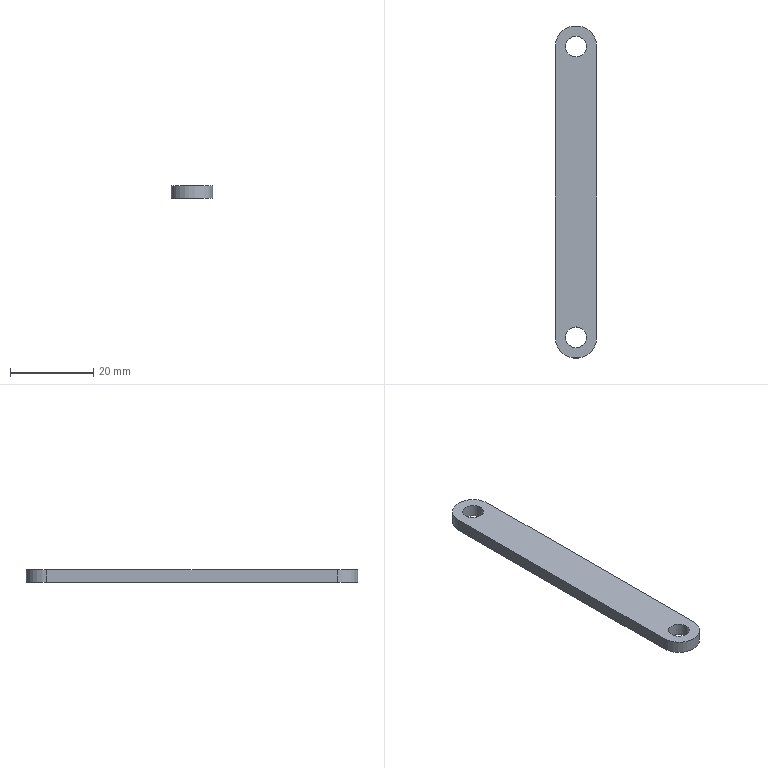Part | STEP file | 1-28.6 | 1 solid | 8 faces | box 10 x 80 x 3 mm | volume 2218 mm3 | plane 4 | cylinder 4 | commonest cylinder face diameters 5 x2 10 x2
STEP:
#1=CARTESIAN_POINT('',(0.,0.,0.));
#2=DIRECTION('',(0.,0.,1.));
#3=DIRECTION('',(1.,0.,0.));
#4=AXIS2_PLACEMENT_3D('',#1,#2,#3);
#5=CARTESIAN_POINT('',(-5.,0.,0.));
#6=VERTEX_POINT('',#5);
#7=CARTESIAN_POINT('',(5.,0.,0.));
#8=VERTEX_POINT('',#7);
#9=CARTESIAN_POINT('',(0.,0.,0.));
#10=DIRECTION('',(0.,0.,1.));
#11=DIRECTION('',(-1.,0.,0.));
#12=AXIS2_PLACEMENT_3D('',#9,#10,#11);
#13=CIRCLE('',#12,5.);
#14=CARTESIAN_POINT('',(-35.,35.,0.));
#15=DIRECTION('',(0.,0.,1.));
#16=DIRECTION('',(0.,1.,0.));
#17=AXIS2_PLACEMENT_3D('',#14,#15,#16);
#18=PLANE('',#17);
#19=CARTESIAN_POINT('',(-35.,-35.));
#20=DIRECTION('',(0.,1.));
#21=AXIS2_PLACEMENT_2D('',#19,#20);
#22=CIRCLE('',#21,5.);
#23=(GEOMETRIC_REPRESENTATION_CONTEXT(2)PARAMETRIC_REPRESENTATION_CONTEXT()REPRESENTATION_CONTEXT('',''));
#24=DEFINITIONAL_REPRESENTATION('',(#22),#23);
#25=PCURVE('',#18,#24);
#26=CARTESIAN_POINT('',(0.,0.,0.));
#27=DIRECTION('',(0.,0.,-1.));
#28=DIRECTION('',(-1.,0.,0.));
#29=AXIS2_PLACEMENT_3D('',#26,#27,#28);
#30=CYLINDRICAL_SURFACE('',#29,5.);
#31=CARTESIAN_POINT('',(6.283,0.));
#32=DIRECTION('',(-1.,0.));
#33=VECTOR('',#32,1.);
#34=LINE('',#31,#33);
#35=(GEOMETRIC_REPRESENTATION_CONTEXT(2)PARAMETRIC_REPRESENTATION_CONTEXT()REPRESENTATION_CONTEXT('',''));
#36=DEFINITIONAL_REPRESENTATION('',(#34),#35);
#37=PCURVE('',#30,#36);
#38=SURFACE_CURVE('',#13,(#25,#37),.PCURVE_S1.);
#39=EDGE_CURVE('',#6,#8,#38,.T.);
#40=ORIENTED_EDGE('',*,*,#39,.T.);
#41=CARTESIAN_POINT('',(5.,70.,0.));
#42=VERTEX_POINT('',#41);
#43=CARTESIAN_POINT('',(5.,0.,0.));
#44=DIRECTION('',(0.,1.,0.));
#45=VECTOR('',#44,1.);
#46=LINE('',#43,#45);
#47=CARTESIAN_POINT('',(-35.,-40.));
#48=DIRECTION('',(1.,0.));
#49=VECTOR('',#48,1.);
#50=LINE('',#47,#49);
#51=(GEOMETRIC_REPRESENTATION_CONTEXT(2)PARAMETRIC_REPRESENTATION_CONTEXT()REPRESENTATION_CONTEXT('',''));
#52=DEFINITIONAL_REPRESENTATION('',(#50),#51);
#53=PCURVE('',#18,#52);
#54=CARTESIAN_POINT('',(5.,35.,-1.5));
#55=DIRECTION('',(-1.,0.,0.));
#56=DIRECTION('',(0.,1.,0.));
#57=AXIS2_PLACEMENT_3D('',#54,#55,#56);
#58=PLANE('',#57);
#59=CARTESIAN_POINT('',(-35.,-1.5));
#60=DIRECTION('',(1.,0.));
#61=VECTOR('',#60,1.);
#62=LINE('',#59,#61);
#63=(GEOMETRIC_REPRESENTATION_CONTEXT(2)PARAMETRIC_REPRESENTATION_CONTEXT()REPRESENTATION_CONTEXT('',''));
#64=DEFINITIONAL_REPRESENTATION('',(#62),#63);
#65=PCURVE('',#58,#64);
#66=SURFACE_CURVE('',#46,(#53,#65),.PCURVE_S1.);
#67=EDGE_CURVE('',#8,#42,#66,.T.);
#68=ORIENTED_EDGE('',*,*,#67,.T.);
#69=CARTESIAN_POINT('',(-5.,70.,0.));
#70=VERTEX_POINT('',#69);
#71=CARTESIAN_POINT('',(0.,70.,0.));
#72=DIRECTION('',(0.,0.,1.));
#73=DIRECTION('',(1.,0.,0.));
#74=AXIS2_PLACEMENT_3D('',#71,#72,#73);
#75=CIRCLE('',#74,5.);
#76=CARTESIAN_POINT('',(35.,-35.));
#77=DIRECTION('',(0.,-1.));
#78=AXIS2_PLACEMENT_2D('',#76,#77);
#79=CIRCLE('',#78,5.);
#80=(GEOMETRIC_REPRESENTATION_CONTEXT(2)PARAMETRIC_REPRESENTATION_CONTEXT()REPRESENTATION_CONTEXT('',''));
#81=DEFINITIONAL_REPRESENTATION('',(#79),#80);
#82=PCURVE('',#18,#81);
#83=CARTESIAN_POINT('',(0.,70.,0.));
#84=DIRECTION('',(0.,0.,-1.));
#85=DIRECTION('',(1.,0.,0.));
#86=AXIS2_PLACEMENT_3D('',#83,#84,#85);
#87=CYLINDRICAL_SURFACE('',#86,5.);
#88=CARTESIAN_POINT('',(6.283,0.));
#89=DIRECTION('',(-1.,0.));
#90=VECTOR('',#89,1.);
#91=LINE('',#88,#90);
#92=(GEOMETRIC_REPRESENTATION_CONTEXT(2)PARAMETRIC_REPRESENTATION_CONTEXT()REPRESENTATION_CONTEXT('',''));
#93=DEFINITIONAL_REPRESENTATION('',(#91),#92);
#94=PCURVE('',#87,#93);
#95=SURFACE_CURVE('',#75,(#82,#94),.PCURVE_S1.);
#96=EDGE_CURVE('',#42,#70,#95,.T.);
#97=ORIENTED_EDGE('',*,*,#96,.T.);
#98=CARTESIAN_POINT('',(-5.,70.,0.));
#99=DIRECTION('',(0.,-1.,0.));
#100=VECTOR('',#99,1.);
#101=LINE('',#98,#100);
#102=CARTESIAN_POINT('',(35.,-30.));
#103=DIRECTION('',(-1.,0.));
#104=VECTOR('',#103,1.);
#105=LINE('',#102,#104);
#106=(GEOMETRIC_REPRESENTATION_CONTEXT(2)PARAMETRIC_REPRESENTATION_CONTEXT()REPRESENTATION_CONTEXT('',''));
#107=DEFINITIONAL_REPRESENTATION('',(#105),#106);
#108=PCURVE('',#18,#107);
#109=CARTESIAN_POINT('',(-5.,35.,-1.5));
#110=DIRECTION('',(1.,0.,0.));
#111=DIRECTION('',(0.,-1.,0.));
#112=AXIS2_PLACEMENT_3D('',#109,#110,#111);
#113=PLANE('',#112);
#114=CARTESIAN_POINT('',(-35.,-1.5));
#115=DIRECTION('',(1.,0.));
#116=VECTOR('',#115,1.);
#117=LINE('',#114,#116);
#118=(GEOMETRIC_REPRESENTATION_CONTEXT(2)PARAMETRIC_REPRESENTATION_CONTEXT()REPRESENTATION_CONTEXT('',''));
#119=DEFINITIONAL_REPRESENTATION('',(#117),#118);
#120=PCURVE('',#113,#119);
#121=SURFACE_CURVE('',#101,(#108,#120),.PCURVE_S1.);
#122=EDGE_CURVE('',#70,#6,#121,.T.);
#123=ORIENTED_EDGE('',*,*,#122,.T.);
#124=EDGE_LOOP('',(#40,#68,#97,#123));
#125=FACE_BOUND('',#124,.T.);
#126=CARTESIAN_POINT('',(0.,2.5,0.));
#127=VERTEX_POINT('',#126);
#128=CARTESIAN_POINT('',(0.,0.,0.));
#129=DIRECTION('',(0.,0.,-1.));
#130=DIRECTION('',(0.,1.,0.));
#131=AXIS2_PLACEMENT_3D('',#128,#129,#130);
#132=CIRCLE('',#131,2.5);
#133=CARTESIAN_POINT('',(-32.5,-35.));
#134=CARTESIAN_POINT('',(-32.5,-39.33));
#135=CARTESIAN_POINT('',(-36.25,-37.165));
#136=CARTESIAN_POINT('',(-40.,-35.));
#137=CARTESIAN_POINT('',(-36.25,-32.835));
#138=CARTESIAN_POINT('',(-32.5,-30.67));
#139=CARTESIAN_POINT('',(-32.5,-35.));
#140=(BOUNDED_CURVE()B_SPLINE_CURVE(2,(#133,#134,#135,#136,#137,#138,#139),.UNSPECIFIED.,.T.,.F.)B_SPLINE_CURVE_WITH_KNOTS((1,2,2,2,2,1),(-2.094,0.,2.094,4.189,6.283,8.378),.UNSPECIFIED.)CURVE()GEOMETRIC_REPRESENTATION_ITEM()RATIONAL_B_SPLINE_CURVE((1.,0.5,1.,0.5,1.,0.5,1.))REPRESENTATION_ITEM(''));
#141=(GEOMETRIC_REPRESENTATION_CONTEXT(2)PARAMETRIC_REPRESENTATION_CONTEXT()REPRESENTATION_CONTEXT('',''));
#142=DEFINITIONAL_REPRESENTATION('',(#140),#141);
#143=PCURVE('',#18,#142);
#144=CARTESIAN_POINT('',(0.,0.,0.));
#145=DIRECTION('',(0.,0.,-1.));
#146=DIRECTION('',(0.,1.,0.));
#147=AXIS2_PLACEMENT_3D('',#144,#145,#146);
#148=CYLINDRICAL_SURFACE('',#147,2.5);
#149=CARTESIAN_POINT('',(0.,0.));
#150=DIRECTION('',(1.,0.));
#151=VECTOR('',#150,1.);
#152=LINE('',#149,#151);
#153=(GEOMETRIC_REPRESENTATION_CONTEXT(2)PARAMETRIC_REPRESENTATION_CONTEXT()REPRESENTATION_CONTEXT('',''));
#154=DEFINITIONAL_REPRESENTATION('',(#152),#153);
#155=PCURVE('',#148,#154);
#156=SURFACE_CURVE('',#132,(#143,#155),.PCURVE_S1.);
#157=EDGE_CURVE('',#127,#127,#156,.T.);
#158=ORIENTED_EDGE('',*,*,#157,.T.);
#159=EDGE_LOOP('',(#158));
#160=FACE_BOUND('',#159,.T.);
#161=CARTESIAN_POINT('',(0.,72.5,0.));
#162=VERTEX_POINT('',#161);
#163=CARTESIAN_POINT('',(0.,70.,0.));
#164=DIRECTION('',(0.,0.,-1.));
#165=DIRECTION('',(0.,1.,0.));
#166=AXIS2_PLACEMENT_3D('',#163,#164,#165);
#167=CIRCLE('',#166,2.5);
#168=CARTESIAN_POINT('',(37.5,-35.));
#169=CARTESIAN_POINT('',(37.5,-39.33));
#170=CARTESIAN_POINT('',(33.75,-37.165));
#171=CARTESIAN_POINT('',(30.,-35.));
#172=CARTESIAN_POINT('',(33.75,-32.835));
#173=CARTESIAN_POINT('',(37.5,-30.67));
#174=CARTESIAN_POINT('',(37.5,-35.));
#175=(BOUNDED_CURVE()B_SPLINE_CURVE(2,(#168,#169,#170,#171,#172,#173,#174),.UNSPECIFIED.,.T.,.F.)B_SPLINE_CURVE_WITH_KNOTS((1,2,2,2,2,1),(-2.094,0.,2.094,4.189,6.283,8.378),.UNSPECIFIED.)CURVE()GEOMETRIC_REPRESENTATION_ITEM()RATIONAL_B_SPLINE_CURVE((1.,0.5,1.,0.5,1.,0.5,1.))REPRESENTATION_ITEM(''));
#176=(GEOMETRIC_REPRESENTATION_CONTEXT(2)PARAMETRIC_REPRESENTATION_CONTEXT()REPRESENTATION_CONTEXT('',''));
#177=DEFINITIONAL_REPRESENTATION('',(#175),#176);
#178=PCURVE('',#18,#177);
#179=CARTESIAN_POINT('',(0.,70.,0.));
#180=DIRECTION('',(0.,0.,-1.));
#181=DIRECTION('',(0.,1.,0.));
#182=AXIS2_PLACEMENT_3D('',#179,#180,#181);
#183=CYLINDRICAL_SURFACE('',#182,2.5);
#184=CARTESIAN_POINT('',(0.,0.));
#185=DIRECTION('',(1.,0.));
#186=VECTOR('',#185,1.);
#187=LINE('',#184,#186);
#188=(GEOMETRIC_REPRESENTATION_CONTEXT(2)PARAMETRIC_REPRESENTATION_CONTEXT()REPRESENTATION_CONTEXT('',''));
#189=DEFINITIONAL_REPRESENTATION('',(#187),#188);
#190=PCURVE('',#183,#189);
#191=SURFACE_CURVE('',#167,(#178,#190),.PCURVE_S1.);
#192=EDGE_CURVE('',#162,#162,#191,.T.);
#193=ORIENTED_EDGE('',*,*,#192,.T.);
#194=EDGE_LOOP('',(#193));
#195=FACE_BOUND('',#194,.T.);
#196=ADVANCED_FACE('',(#125,#160,#195),#18,.T.);
#197=CARTESIAN_POINT('',(-5.,0.,-3.));
#198=VERTEX_POINT('',#197);
#199=CARTESIAN_POINT('',(5.,0.,-3.));
#200=VERTEX_POINT('',#199);
#201=CARTESIAN_POINT('',(0.,0.,-3.));
#202=DIRECTION('',(0.,0.,1.));
#203=DIRECTION('',(-1.,0.,0.));
#204=AXIS2_PLACEMENT_3D('',#201,#202,#203);
#205=CIRCLE('',#204,5.);
#206=CARTESIAN_POINT('',(-35.,35.,-3.));
#207=DIRECTION('',(0.,0.,1.));
#208=DIRECTION('',(0.,1.,0.));
#209=AXIS2_PLACEMENT_3D('',#206,#207,#208);
#210=PLANE('',#209);
#211=CARTESIAN_POINT('',(-35.,-35.));
#212=DIRECTION('',(0.,1.));
#213=AXIS2_PLACEMENT_2D('',#211,#212);
#214=CIRCLE('',#213,5.);
#215=(GEOMETRIC_REPRESENTATION_CONTEXT(2)PARAMETRIC_REPRESENTATION_CONTEXT()REPRESENTATION_CONTEXT('',''));
#216=DEFINITIONAL_REPRESENTATION('',(#214),#215);
#217=PCURVE('',#210,#216);
#218=CARTESIAN_POINT('',(6.283,3.));
#219=DIRECTION('',(-1.,0.));
#220=VECTOR('',#219,1.);
#221=LINE('',#218,#220);
#222=(GEOMETRIC_REPRESENTATION_CONTEXT(2)PARAMETRIC_REPRESENTATION_CONTEXT()REPRESENTATION_CONTEXT('',''));
#223=DEFINITIONAL_REPRESENTATION('',(#221),#222);
#224=PCURVE('',#30,#223);
#225=SURFACE_CURVE('',#205,(#217,#224),.PCURVE_S1.);
#226=EDGE_CURVE('',#198,#200,#225,.T.);
#227=ORIENTED_EDGE('',*,*,#226,.T.);
#228=CARTESIAN_POINT('',(5.,70.,-3.));
#229=VERTEX_POINT('',#228);
#230=CARTESIAN_POINT('',(5.,0.,-3.));
#231=DIRECTION('',(0.,1.,0.));
#232=VECTOR('',#231,1.);
#233=LINE('',#230,#232);
#234=CARTESIAN_POINT('',(-35.,-40.));
#235=DIRECTION('',(1.,0.));
#236=VECTOR('',#235,1.);
#237=LINE('',#234,#236);
#238=(GEOMETRIC_REPRESENTATION_CONTEXT(2)PARAMETRIC_REPRESENTATION_CONTEXT()REPRESENTATION_CONTEXT('',''));
#239=DEFINITIONAL_REPRESENTATION('',(#237),#238);
#240=PCURVE('',#210,#239);
#241=CARTESIAN_POINT('',(-35.,1.5));
#242=DIRECTION('',(1.,0.));
#243=VECTOR('',#242,1.);
#244=LINE('',#241,#243);
#245=(GEOMETRIC_REPRESENTATION_CONTEXT(2)PARAMETRIC_REPRESENTATION_CONTEXT()REPRESENTATION_CONTEXT('',''));
#246=DEFINITIONAL_REPRESENTATION('',(#244),#245);
#247=PCURVE('',#58,#246);
#248=SURFACE_CURVE('',#233,(#240,#247),.PCURVE_S1.);
#249=EDGE_CURVE('',#200,#229,#248,.T.);
#250=ORIENTED_EDGE('',*,*,#249,.T.);
#251=CARTESIAN_POINT('',(-5.,70.,-3.));
#252=VERTEX_POINT('',#251);
#253=CARTESIAN_POINT('',(0.,70.,-3.));
#254=DIRECTION('',(0.,0.,1.));
#255=DIRECTION('',(1.,0.,0.));
#256=AXIS2_PLACEMENT_3D('',#253,#254,#255);
#257=CIRCLE('',#256,5.);
#258=CARTESIAN_POINT('',(35.,-35.));
#259=DIRECTION('',(0.,-1.));
#260=AXIS2_PLACEMENT_2D('',#258,#259);
#261=CIRCLE('',#260,5.);
#262=(GEOMETRIC_REPRESENTATION_CONTEXT(2)PARAMETRIC_REPRESENTATION_CONTEXT()REPRESENTATION_CONTEXT('',''));
#263=DEFINITIONAL_REPRESENTATION('',(#261),#262);
#264=PCURVE('',#210,#263);
#265=CARTESIAN_POINT('',(6.283,3.));
#266=DIRECTION('',(-1.,0.));
#267=VECTOR('',#266,1.);
#268=LINE('',#265,#267);
#269=(GEOMETRIC_REPRESENTATION_CONTEXT(2)PARAMETRIC_REPRESENTATION_CONTEXT()REPRESENTATION_CONTEXT('',''));
#270=DEFINITIONAL_REPRESENTATION('',(#268),#269);
#271=PCURVE('',#87,#270);
#272=SURFACE_CURVE('',#257,(#264,#271),.PCURVE_S1.);
#273=EDGE_CURVE('',#229,#252,#272,.T.);
#274=ORIENTED_EDGE('',*,*,#273,.T.);
#275=CARTESIAN_POINT('',(-5.,70.,-3.));
#276=DIRECTION('',(0.,-1.,0.));
#277=VECTOR('',#276,1.);
#278=LINE('',#275,#277);
#279=CARTESIAN_POINT('',(35.,-30.));
#280=DIRECTION('',(-1.,0.));
#281=VECTOR('',#280,1.);
#282=LINE('',#279,#281);
#283=(GEOMETRIC_REPRESENTATION_CONTEXT(2)PARAMETRIC_REPRESENTATION_CONTEXT()REPRESENTATION_CONTEXT('',''));
#284=DEFINITIONAL_REPRESENTATION('',(#282),#283);
#285=PCURVE('',#210,#284);
#286=CARTESIAN_POINT('',(-35.,1.5));
#287=DIRECTION('',(1.,0.));
#288=VECTOR('',#287,1.);
#289=LINE('',#286,#288);
#290=(GEOMETRIC_REPRESENTATION_CONTEXT(2)PARAMETRIC_REPRESENTATION_CONTEXT()REPRESENTATION_CONTEXT('',''));
#291=DEFINITIONAL_REPRESENTATION('',(#289),#290);
#292=PCURVE('',#113,#291);
#293=SURFACE_CURVE('',#278,(#285,#292),.PCURVE_S1.);
#294=EDGE_CURVE('',#252,#198,#293,.T.);
#295=ORIENTED_EDGE('',*,*,#294,.T.);
#296=EDGE_LOOP('',(#227,#250,#274,#295));
#297=FACE_BOUND('',#296,.F.);
#298=CARTESIAN_POINT('',(0.,2.5,-3.));
#299=VERTEX_POINT('',#298);
#300=CARTESIAN_POINT('',(0.,0.,-3.));
#301=DIRECTION('',(0.,0.,-1.));
#302=DIRECTION('',(0.,1.,0.));
#303=AXIS2_PLACEMENT_3D('',#300,#301,#302);
#304=CIRCLE('',#303,2.5);
#305=CARTESIAN_POINT('',(-32.5,-35.));
#306=CARTESIAN_POINT('',(-32.5,-39.33));
#307=CARTESIAN_POINT('',(-36.25,-37.165));
#308=CARTESIAN_POINT('',(-40.,-35.));
#309=CARTESIAN_POINT('',(-36.25,-32.835));
#310=CARTESIAN_POINT('',(-32.5,-30.67));
#311=CARTESIAN_POINT('',(-32.5,-35.));
#312=(BOUNDED_CURVE()B_SPLINE_CURVE(2,(#305,#306,#307,#308,#309,#310,#311),.UNSPECIFIED.,.T.,.F.)B_SPLINE_CURVE_WITH_KNOTS((1,2,2,2,2,1),(-2.094,0.,2.094,4.189,6.283,8.378),.UNSPECIFIED.)CURVE()GEOMETRIC_REPRESENTATION_ITEM()RATIONAL_B_SPLINE_CURVE((1.,0.5,1.,0.5,1.,0.5,1.))REPRESENTATION_ITEM(''));
#313=(GEOMETRIC_REPRESENTATION_CONTEXT(2)PARAMETRIC_REPRESENTATION_CONTEXT()REPRESENTATION_CONTEXT('',''));
#314=DEFINITIONAL_REPRESENTATION('',(#312),#313);
#315=PCURVE('',#210,#314);
#316=CARTESIAN_POINT('',(0.,3.));
#317=DIRECTION('',(1.,0.));
#318=VECTOR('',#317,1.);
#319=LINE('',#316,#318);
#320=(GEOMETRIC_REPRESENTATION_CONTEXT(2)PARAMETRIC_REPRESENTATION_CONTEXT()REPRESENTATION_CONTEXT('',''));
#321=DEFINITIONAL_REPRESENTATION('',(#319),#320);
#322=PCURVE('',#148,#321);
#323=SURFACE_CURVE('',#304,(#315,#322),.PCURVE_S1.);
#324=EDGE_CURVE('',#299,#299,#323,.T.);
#325=ORIENTED_EDGE('',*,*,#324,.T.);
#326=EDGE_LOOP('',(#325));
#327=FACE_BOUND('',#326,.F.);
#328=CARTESIAN_POINT('',(0.,72.5,-3.));
#329=VERTEX_POINT('',#328);
#330=CARTESIAN_POINT('',(0.,70.,-3.));
#331=DIRECTION('',(0.,0.,-1.));
#332=DIRECTION('',(0.,1.,0.));
#333=AXIS2_PLACEMENT_3D('',#330,#331,#332);
#334=CIRCLE('',#333,2.5);
#335=CARTESIAN_POINT('',(37.5,-35.));
#336=CARTESIAN_POINT('',(37.5,-39.33));
#337=CARTESIAN_POINT('',(33.75,-37.165));
#338=CARTESIAN_POINT('',(30.,-35.));
#339=CARTESIAN_POINT('',(33.75,-32.835));
#340=CARTESIAN_POINT('',(37.5,-30.67));
#341=CARTESIAN_POINT('',(37.5,-35.));
#342=(BOUNDED_CURVE()B_SPLINE_CURVE(2,(#335,#336,#337,#338,#339,#340,#341),.UNSPECIFIED.,.T.,.F.)B_SPLINE_CURVE_WITH_KNOTS((1,2,2,2,2,1),(-2.094,0.,2.094,4.189,6.283,8.378),.UNSPECIFIED.)CURVE()GEOMETRIC_REPRESENTATION_ITEM()RATIONAL_B_SPLINE_CURVE((1.,0.5,1.,0.5,1.,0.5,1.))REPRESENTATION_ITEM(''));
#343=(GEOMETRIC_REPRESENTATION_CONTEXT(2)PARAMETRIC_REPRESENTATION_CONTEXT()REPRESENTATION_CONTEXT('',''));
#344=DEFINITIONAL_REPRESENTATION('',(#342),#343);
#345=PCURVE('',#210,#344);
#346=CARTESIAN_POINT('',(0.,3.));
#347=DIRECTION('',(1.,0.));
#348=VECTOR('',#347,1.);
#349=LINE('',#346,#348);
#350=(GEOMETRIC_REPRESENTATION_CONTEXT(2)PARAMETRIC_REPRESENTATION_CONTEXT()REPRESENTATION_CONTEXT('',''));
#351=DEFINITIONAL_REPRESENTATION('',(#349),#350);
#352=PCURVE('',#183,#351);
#353=SURFACE_CURVE('',#334,(#345,#352),.PCURVE_S1.);
#354=EDGE_CURVE('',#329,#329,#353,.T.);
#355=ORIENTED_EDGE('',*,*,#354,.T.);
#356=EDGE_LOOP('',(#355));
#357=FACE_BOUND('',#356,.F.);
#358=ADVANCED_FACE('',(#297,#327,#357),#210,.F.);
#359=CARTESIAN_POINT('',(-5.,0.,0.));
#360=DIRECTION('',(0.,0.,-1.));
#361=VECTOR('',#360,1.);
#362=LINE('',#359,#361);
#363=CARTESIAN_POINT('',(6.283,0.));
#364=DIRECTION('',(0.,1.));
#365=VECTOR('',#364,1.);
#366=LINE('',#363,#365);
#367=(GEOMETRIC_REPRESENTATION_CONTEXT(2)PARAMETRIC_REPRESENTATION_CONTEXT()REPRESENTATION_CONTEXT('',''));
#368=DEFINITIONAL_REPRESENTATION('',(#366),#367);
#369=PCURVE('',#30,#368);
#370=CARTESIAN_POINT('',(35.,-1.5));
#371=DIRECTION('',(0.,1.));
#372=VECTOR('',#371,1.);
#373=LINE('',#370,#372);
#374=(GEOMETRIC_REPRESENTATION_CONTEXT(2)PARAMETRIC_REPRESENTATION_CONTEXT()REPRESENTATION_CONTEXT('',''));
#375=DEFINITIONAL_REPRESENTATION('',(#373),#374);
#376=PCURVE('',#113,#375);
#377=SURFACE_CURVE('',#362,(#369,#376),.PCURVE_S1.);
#378=EDGE_CURVE('',#6,#198,#377,.T.);
#379=ORIENTED_EDGE('',*,*,#378,.T.);
#380=ORIENTED_EDGE('',*,*,#226,.T.);
#381=CARTESIAN_POINT('',(5.,0.,0.));
#382=DIRECTION('',(0.,0.,-1.));
#383=VECTOR('',#382,1.);
#384=LINE('',#381,#383);
#385=CARTESIAN_POINT('',(3.142,0.));
#386=DIRECTION('',(0.,1.));
#387=VECTOR('',#386,1.);
#388=LINE('',#385,#387);
#389=(GEOMETRIC_REPRESENTATION_CONTEXT(2)PARAMETRIC_REPRESENTATION_CONTEXT()REPRESENTATION_CONTEXT('',''));
#390=DEFINITIONAL_REPRESENTATION('',(#388),#389);
#391=PCURVE('',#30,#390);
#392=CARTESIAN_POINT('',(-35.,-1.5));
#393=DIRECTION('',(0.,1.));
#394=VECTOR('',#393,1.);
#395=LINE('',#392,#394);
#396=(GEOMETRIC_REPRESENTATION_CONTEXT(2)PARAMETRIC_REPRESENTATION_CONTEXT()REPRESENTATION_CONTEXT('',''));
#397=DEFINITIONAL_REPRESENTATION('',(#395),#396);
#398=PCURVE('',#58,#397);
#399=SURFACE_CURVE('',#384,(#391,#398),.PCURVE_S1.);
#400=EDGE_CURVE('',#8,#200,#399,.T.);
#401=ORIENTED_EDGE('',*,*,#400,.F.);
#402=ORIENTED_EDGE('',*,*,#39,.F.);
#403=EDGE_LOOP('',(#379,#380,#401,#402));
#404=FACE_BOUND('',#403,.T.);
#405=ADVANCED_FACE('',(#404),#30,.T.);
#406=ORIENTED_EDGE('',*,*,#67,.T.);
#407=CARTESIAN_POINT('',(5.,70.,0.));
#408=DIRECTION('',(0.,0.,-1.));
#409=VECTOR('',#408,1.);
#410=LINE('',#407,#409);
#411=CARTESIAN_POINT('',(35.,-1.5));
#412=DIRECTION('',(0.,1.));
#413=VECTOR('',#412,1.);
#414=LINE('',#411,#413);
#415=(GEOMETRIC_REPRESENTATION_CONTEXT(2)PARAMETRIC_REPRESENTATION_CONTEXT()REPRESENTATION_CONTEXT('',''));
#416=DEFINITIONAL_REPRESENTATION('',(#414),#415);
#417=PCURVE('',#58,#416);
#418=CARTESIAN_POINT('',(6.283,0.));
#419=DIRECTION('',(0.,1.));
#420=VECTOR('',#419,1.);
#421=LINE('',#418,#420);
#422=(GEOMETRIC_REPRESENTATION_CONTEXT(2)PARAMETRIC_REPRESENTATION_CONTEXT()REPRESENTATION_CONTEXT('',''));
#423=DEFINITIONAL_REPRESENTATION('',(#421),#422);
#424=PCURVE('',#87,#423);
#425=SURFACE_CURVE('',#410,(#417,#424),.PCURVE_S1.);
#426=EDGE_CURVE('',#42,#229,#425,.T.);
#427=ORIENTED_EDGE('',*,*,#426,.T.);
#428=ORIENTED_EDGE('',*,*,#249,.F.);
#429=ORIENTED_EDGE('',*,*,#400,.F.);
#430=EDGE_LOOP('',(#406,#427,#428,#429));
#431=FACE_BOUND('',#430,.F.);
#432=ADVANCED_FACE('',(#431),#58,.F.);
#433=ORIENTED_EDGE('',*,*,#426,.T.);
#434=ORIENTED_EDGE('',*,*,#273,.T.);
#435=CARTESIAN_POINT('',(-5.,70.,0.));
#436=DIRECTION('',(0.,0.,-1.));
#437=VECTOR('',#436,1.);
#438=LINE('',#435,#437);
#439=CARTESIAN_POINT('',(3.142,0.));
#440=DIRECTION('',(0.,1.));
#441=VECTOR('',#440,1.);
#442=LINE('',#439,#441);
#443=(GEOMETRIC_REPRESENTATION_CONTEXT(2)PARAMETRIC_REPRESENTATION_CONTEXT()REPRESENTATION_CONTEXT('',''));
#444=DEFINITIONAL_REPRESENTATION('',(#442),#443);
#445=PCURVE('',#87,#444);
#446=CARTESIAN_POINT('',(-35.,-1.5));
#447=DIRECTION('',(0.,1.));
#448=VECTOR('',#447,1.);
#449=LINE('',#446,#448);
#450=(GEOMETRIC_REPRESENTATION_CONTEXT(2)PARAMETRIC_REPRESENTATION_CONTEXT()REPRESENTATION_CONTEXT('',''));
#451=DEFINITIONAL_REPRESENTATION('',(#449),#450);
#452=PCURVE('',#113,#451);
#453=SURFACE_CURVE('',#438,(#445,#452),.PCURVE_S1.);
#454=EDGE_CURVE('',#70,#252,#453,.T.);
#455=ORIENTED_EDGE('',*,*,#454,.F.);
#456=ORIENTED_EDGE('',*,*,#96,.F.);
#457=EDGE_LOOP('',(#433,#434,#455,#456));
#458=FACE_BOUND('',#457,.T.);
#459=ADVANCED_FACE('',(#458),#87,.T.);
#460=ORIENTED_EDGE('',*,*,#122,.T.);
#461=ORIENTED_EDGE('',*,*,#378,.T.);
#462=ORIENTED_EDGE('',*,*,#294,.F.);
#463=ORIENTED_EDGE('',*,*,#454,.F.);
#464=EDGE_LOOP('',(#460,#461,#462,#463));
#465=FACE_BOUND('',#464,.F.);
#466=ADVANCED_FACE('',(#465),#113,.F.);
#467=ORIENTED_EDGE('',*,*,#157,.T.);
#468=CARTESIAN_POINT('',(0.,2.5,0.));
#469=DIRECTION('',(0.,0.,-1.));
#470=VECTOR('',#469,1.);
#471=LINE('',#468,#470);
#472=CARTESIAN_POINT('',(6.283,0.));
#473=DIRECTION('',(0.,1.));
#474=VECTOR('',#473,1.);
#475=LINE('',#472,#474);
#476=(GEOMETRIC_REPRESENTATION_CONTEXT(2)PARAMETRIC_REPRESENTATION_CONTEXT()REPRESENTATION_CONTEXT('',''));
#477=DEFINITIONAL_REPRESENTATION('',(#475),#476);
#478=PCURVE('',#148,#477);
#479=CARTESIAN_POINT('',(0.,0.));
#480=DIRECTION('',(0.,1.));
#481=VECTOR('',#480,1.);
#482=LINE('',#479,#481);
#483=(GEOMETRIC_REPRESENTATION_CONTEXT(2)PARAMETRIC_REPRESENTATION_CONTEXT()REPRESENTATION_CONTEXT('',''));
#484=DEFINITIONAL_REPRESENTATION('',(#482),#483);
#485=PCURVE('',#148,#484);
#486=SEAM_CURVE('',#471,(#478,#485),.PCURVE_S1.);
#487=EDGE_CURVE('',#127,#299,#486,.T.);
#488=ORIENTED_EDGE('',*,*,#487,.T.);
#489=ORIENTED_EDGE('',*,*,#324,.F.);
#490=ORIENTED_EDGE('',*,*,#487,.F.);
#491=EDGE_LOOP('',(#467,#488,#489,#490));
#492=FACE_BOUND('',#491,.F.);
#493=ADVANCED_FACE('',(#492),#148,.F.);
#494=ORIENTED_EDGE('',*,*,#192,.T.);
#495=CARTESIAN_POINT('',(0.,72.5,0.));
#496=DIRECTION('',(0.,0.,-1.));
#497=VECTOR('',#496,1.);
#498=LINE('',#495,#497);
#499=CARTESIAN_POINT('',(6.283,0.));
#500=DIRECTION('',(0.,1.));
#501=VECTOR('',#500,1.);
#502=LINE('',#499,#501);
#503=(GEOMETRIC_REPRESENTATION_CONTEXT(2)PARAMETRIC_REPRESENTATION_CONTEXT()REPRESENTATION_CONTEXT('',''));
#504=DEFINITIONAL_REPRESENTATION('',(#502),#503);
#505=PCURVE('',#183,#504);
#506=CARTESIAN_POINT('',(0.,0.));
#507=DIRECTION('',(0.,1.));
#508=VECTOR('',#507,1.);
#509=LINE('',#506,#508);
#510=(GEOMETRIC_REPRESENTATION_CONTEXT(2)PARAMETRIC_REPRESENTATION_CONTEXT()REPRESENTATION_CONTEXT('',''));
#511=DEFINITIONAL_REPRESENTATION('',(#509),#510);
#512=PCURVE('',#183,#511);
#513=SEAM_CURVE('',#498,(#505,#512),.PCURVE_S1.);
#514=EDGE_CURVE('',#162,#329,#513,.T.);
#515=ORIENTED_EDGE('',*,*,#514,.T.);
#516=ORIENTED_EDGE('',*,*,#354,.F.);
#517=ORIENTED_EDGE('',*,*,#514,.F.);
#518=EDGE_LOOP('',(#494,#515,#516,#517));
#519=FACE_BOUND('',#518,.F.);
#520=ADVANCED_FACE('',(#519),#183,.F.);
#521=CLOSED_SHELL('',(#196,#358,#405,#432,#459,#466,#493,#520));
#522=MANIFOLD_SOLID_BREP('',#521);
#523=(LENGTH_UNIT()NAMED_UNIT(*)SI_UNIT(.MILLI.,.METRE.));
#524=UNCERTAINTY_MEASURE_WITH_UNIT(LENGTH_MEASURE(0.0000001),#523,'','');
#525=(NAMED_UNIT(*)PLANE_ANGLE_UNIT()SI_UNIT($,.RADIAN.));
#526=(NAMED_UNIT(*)SI_UNIT($,.STERADIAN.)SOLID_ANGLE_UNIT());
#527=(GEOMETRIC_REPRESENTATION_CONTEXT(3)GLOBAL_UNCERTAINTY_ASSIGNED_CONTEXT((#524))GLOBAL_UNIT_ASSIGNED_CONTEXT((#523,#525,#526))REPRESENTATION_CONTEXT('',''));
#528=ADVANCED_BREP_SHAPE_REPRESENTATION('',(#4,#522),#527);